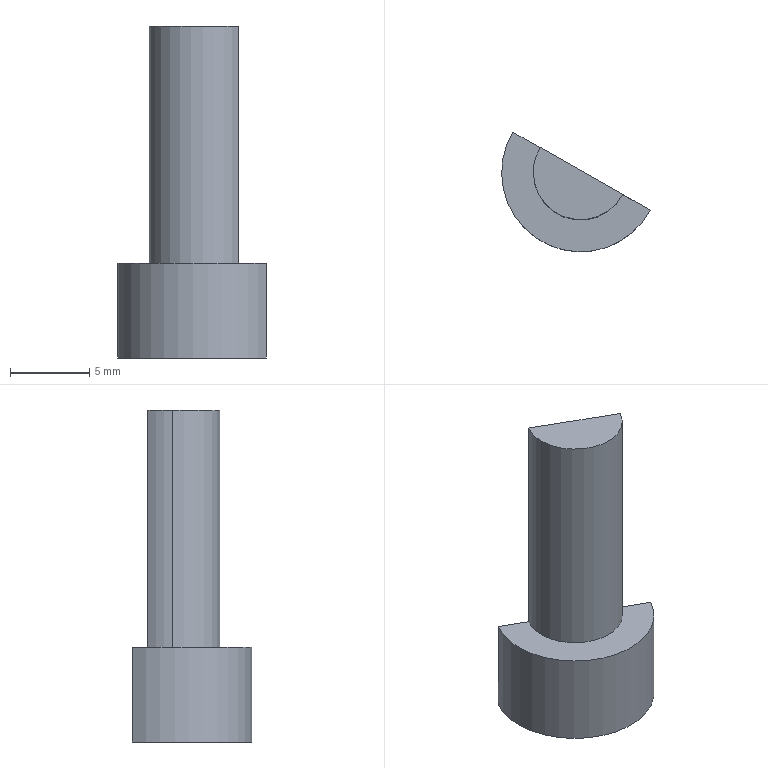Part | STEP file | LG M6_1.5F | 1 solid | 12 faces | box 9.402 x 7.564 x 21 mm | volume 429.881 mm3 | plane 9 | cylinder 3 | commonest cylinder face diameters 6 x2 10 x1
STEP:
#1=CARTESIAN_POINT('',(0.,0.,0.));
#2=DIRECTION('',(0.,0.,1.));
#3=DIRECTION('',(1.,0.,0.));
#4=AXIS2_PLACEMENT_3D('',#1,#2,#3);
#5=CARTESIAN_POINT('',(-3.,0.,15.));
#6=VERTEX_POINT('',#5);
#7=CARTESIAN_POINT('',(2.662,-1.383,15.));
#8=VERTEX_POINT('',#7);
#9=CARTESIAN_POINT('',(0.,0.,15.));
#10=DIRECTION('',(0.,0.,1.));
#11=DIRECTION('',(1.,0.,0.));
#12=AXIS2_PLACEMENT_3D('',#9,#10,#11);
#13=CIRCLE('',#12,3.);
#14=CARTESIAN_POINT('',(0.,0.,15.));
#15=DIRECTION('',(0.,0.,-1.));
#16=DIRECTION('',(-1.,0.,0.));
#17=AXIS2_PLACEMENT_3D('',#14,#15,#16);
#18=CYLINDRICAL_SURFACE('',#17,3.);
#19=CARTESIAN_POINT('',(9.425,0.));
#20=DIRECTION('',(-1.,0.));
#21=VECTOR('',#20,1.);
#22=LINE('',#19,#21);
#23=(GEOMETRIC_REPRESENTATION_CONTEXT(2)PARAMETRIC_REPRESENTATION_CONTEXT()REPRESENTATION_CONTEXT('',''));
#24=DEFINITIONAL_REPRESENTATION('',(#22),#23);
#25=PCURVE('',#18,#24);
#26=CARTESIAN_POINT('',(0.,0.,15.));
#27=DIRECTION('',(0.,0.,1.));
#28=DIRECTION('',(1.,0.,0.));
#29=AXIS2_PLACEMENT_3D('',#26,#27,#28);
#30=PLANE('',#29);
#31=CARTESIAN_POINT('',(0.,0.));
#32=DIRECTION('',(1.,0.));
#33=AXIS2_PLACEMENT_2D('',#31,#32);
#34=CIRCLE('',#33,3.);
#35=(GEOMETRIC_REPRESENTATION_CONTEXT(2)PARAMETRIC_REPRESENTATION_CONTEXT()REPRESENTATION_CONTEXT('',''));
#36=DEFINITIONAL_REPRESENTATION('',(#34),#35);
#37=PCURVE('',#30,#36);
#38=SURFACE_CURVE('',#13,(#25,#37),.PCURVE_S1.);
#39=EDGE_CURVE('',#6,#8,#38,.T.);
#40=ORIENTED_EDGE('',*,*,#39,.F.);
#41=CARTESIAN_POINT('',(-3.,0.,0.));
#42=VERTEX_POINT('',#41);
#43=CARTESIAN_POINT('',(-3.,0.,15.));
#44=DIRECTION('',(0.,0.,-1.));
#45=VECTOR('',#44,1.);
#46=LINE('',#43,#45);
#47=CARTESIAN_POINT('',(6.283,0.));
#48=DIRECTION('',(0.,1.));
#49=VECTOR('',#48,1.);
#50=LINE('',#47,#49);
#51=(GEOMETRIC_REPRESENTATION_CONTEXT(2)PARAMETRIC_REPRESENTATION_CONTEXT()REPRESENTATION_CONTEXT('',''));
#52=DEFINITIONAL_REPRESENTATION('',(#50),#51);
#53=PCURVE('',#18,#52);
#54=CARTESIAN_POINT('',(0.,0.,15.));
#55=DIRECTION('',(0.,0.,-1.));
#56=DIRECTION('',(-1.,0.,0.));
#57=AXIS2_PLACEMENT_3D('',#54,#55,#56);
#58=CYLINDRICAL_SURFACE('',#57,3.);
#59=CARTESIAN_POINT('',(0.,0.));
#60=DIRECTION('',(0.,1.));
#61=VECTOR('',#60,1.);
#62=LINE('',#59,#61);
#63=(GEOMETRIC_REPRESENTATION_CONTEXT(2)PARAMETRIC_REPRESENTATION_CONTEXT()REPRESENTATION_CONTEXT('',''));
#64=DEFINITIONAL_REPRESENTATION('',(#62),#63);
#65=PCURVE('',#58,#64);
#66=SURFACE_CURVE('',#46,(#53,#65),.PCURVE_S1.);
#67=EDGE_CURVE('',#6,#42,#66,.T.);
#68=ORIENTED_EDGE('',*,*,#67,.T.);
#69=CARTESIAN_POINT('',(2.662,-1.383,0.));
#70=VERTEX_POINT('',#69);
#71=CARTESIAN_POINT('',(0.,0.,0.));
#72=DIRECTION('',(0.,0.,1.));
#73=DIRECTION('',(1.,0.,0.));
#74=AXIS2_PLACEMENT_3D('',#71,#72,#73);
#75=CIRCLE('',#74,3.);
#76=CARTESIAN_POINT('',(9.425,15.));
#77=DIRECTION('',(-1.,0.));
#78=VECTOR('',#77,1.);
#79=LINE('',#76,#78);
#80=(GEOMETRIC_REPRESENTATION_CONTEXT(2)PARAMETRIC_REPRESENTATION_CONTEXT()REPRESENTATION_CONTEXT('',''));
#81=DEFINITIONAL_REPRESENTATION('',(#79),#80);
#82=PCURVE('',#18,#81);
#83=CARTESIAN_POINT('',(0.,0.,0.));
#84=DIRECTION('',(0.,0.,1.));
#85=DIRECTION('',(1.,0.,0.));
#86=AXIS2_PLACEMENT_3D('',#83,#84,#85);
#87=PLANE('',#86);
#88=CARTESIAN_POINT('',(0.,0.));
#89=DIRECTION('',(1.,0.));
#90=AXIS2_PLACEMENT_2D('',#88,#89);
#91=CIRCLE('',#90,3.);
#92=(GEOMETRIC_REPRESENTATION_CONTEXT(2)PARAMETRIC_REPRESENTATION_CONTEXT()REPRESENTATION_CONTEXT('',''));
#93=DEFINITIONAL_REPRESENTATION('',(#91),#92);
#94=PCURVE('',#87,#93);
#95=SURFACE_CURVE('',#75,(#82,#94),.PCURVE_S1.);
#96=EDGE_CURVE('',#42,#70,#95,.T.);
#97=ORIENTED_EDGE('',*,*,#96,.T.);
#98=CARTESIAN_POINT('',(2.662,-1.383,15.));
#99=DIRECTION('',(0.,0.,1.));
#100=VECTOR('',#99,1.);
#101=LINE('',#98,#100);
#102=CARTESIAN_POINT('',(3.621,0.));
#103=DIRECTION('',(0.,-1.));
#104=VECTOR('',#103,1.);
#105=LINE('',#102,#104);
#106=(GEOMETRIC_REPRESENTATION_CONTEXT(2)PARAMETRIC_REPRESENTATION_CONTEXT()REPRESENTATION_CONTEXT('',''));
#107=DEFINITIONAL_REPRESENTATION('',(#105),#106);
#108=PCURVE('',#18,#107);
#109=CARTESIAN_POINT('',(312.967,-177.494,-20.57));
#110=DIRECTION('',(-0.4936,-0.8697,0.));
#111=DIRECTION('',(0.8697,-0.4936,0.));
#112=AXIS2_PLACEMENT_3D('',#109,#110,#111);
#113=PLANE('',#112);
#114=CARTESIAN_POINT('',(-356.797,35.57));
#115=DIRECTION('',(0.,1.));
#116=VECTOR('',#115,1.);
#117=LINE('',#114,#116);
#118=(GEOMETRIC_REPRESENTATION_CONTEXT(2)PARAMETRIC_REPRESENTATION_CONTEXT()REPRESENTATION_CONTEXT('',''));
#119=DEFINITIONAL_REPRESENTATION('',(#117),#118);
#120=PCURVE('',#113,#119);
#121=SURFACE_CURVE('',#101,(#108,#120),.PCURVE_S1.);
#122=EDGE_CURVE('',#70,#8,#121,.T.);
#123=ORIENTED_EDGE('',*,*,#122,.T.);
#124=EDGE_LOOP('',(#40,#68,#97,#123));
#125=FACE_BOUND('',#124,.T.);
#126=ADVANCED_FACE('',(#125),#18,.T.);
#127=CARTESIAN_POINT('',(-4.293,2.564,0.));
#128=VERTEX_POINT('',#127);
#129=CARTESIAN_POINT('',(-2.553,1.576,0.));
#130=VERTEX_POINT('',#129);
#131=CARTESIAN_POINT('',(0.05466,0.09631,0.));
#132=DIRECTION('',(0.8697,-0.4936,0.));
#133=VECTOR('',#132,1.);
#134=LINE('',#131,#133);
#135=CARTESIAN_POINT('',(0.05466,0.09631));
#136=DIRECTION('',(0.8697,-0.4936));
#137=VECTOR('',#136,1.);
#138=LINE('',#135,#137);
#139=(GEOMETRIC_REPRESENTATION_CONTEXT(2)PARAMETRIC_REPRESENTATION_CONTEXT()REPRESENTATION_CONTEXT('',''));
#140=DEFINITIONAL_REPRESENTATION('',(#138),#139);
#141=PCURVE('',#87,#140);
#142=CARTESIAN_POINT('',(-359.795,20.57));
#143=DIRECTION('',(1.,0.));
#144=VECTOR('',#143,1.);
#145=LINE('',#142,#144);
#146=(GEOMETRIC_REPRESENTATION_CONTEXT(2)PARAMETRIC_REPRESENTATION_CONTEXT()REPRESENTATION_CONTEXT('',''));
#147=DEFINITIONAL_REPRESENTATION('',(#145),#146);
#148=PCURVE('',#113,#147);
#149=SURFACE_CURVE('',#134,(#141,#148),.PCURVE_S1.);
#150=EDGE_CURVE('',#128,#130,#149,.T.);
#151=ORIENTED_EDGE('',*,*,#150,.F.);
#152=CARTESIAN_POINT('',(4.402,-2.371,0.));
#153=VERTEX_POINT('',#152);
#154=CARTESIAN_POINT('',(0.,0.,0.));
#155=DIRECTION('',(0.,0.,1.));
#156=DIRECTION('',(1.,0.,0.));
#157=AXIS2_PLACEMENT_3D('',#154,#155,#156);
#158=CIRCLE('',#157,5.);
#159=CARTESIAN_POINT('',(0.,0.));
#160=DIRECTION('',(1.,0.));
#161=AXIS2_PLACEMENT_2D('',#159,#160);
#162=CIRCLE('',#161,5.);
#163=(GEOMETRIC_REPRESENTATION_CONTEXT(2)PARAMETRIC_REPRESENTATION_CONTEXT()REPRESENTATION_CONTEXT('',''));
#164=DEFINITIONAL_REPRESENTATION('',(#162),#163);
#165=PCURVE('',#87,#164);
#166=CARTESIAN_POINT('',(0.,0.,-6.));
#167=DIRECTION('',(0.,0.,1.));
#168=DIRECTION('',(1.,0.,0.));
#169=AXIS2_PLACEMENT_3D('',#166,#167,#168);
#170=CYLINDRICAL_SURFACE('',#169,5.);
#171=CARTESIAN_POINT('',(0.,6.));
#172=DIRECTION('',(1.,0.));
#173=VECTOR('',#172,1.);
#174=LINE('',#171,#173);
#175=(GEOMETRIC_REPRESENTATION_CONTEXT(2)PARAMETRIC_REPRESENTATION_CONTEXT()REPRESENTATION_CONTEXT('',''));
#176=DEFINITIONAL_REPRESENTATION('',(#174),#175);
#177=PCURVE('',#170,#176);
#178=SURFACE_CURVE('',#158,(#165,#177),.PCURVE_S1.);
#179=EDGE_CURVE('',#128,#153,#178,.T.);
#180=ORIENTED_EDGE('',*,*,#179,.T.);
#181=CARTESIAN_POINT('',(0.05466,0.09631,0.));
#182=DIRECTION('',(0.8697,-0.4936,0.));
#183=VECTOR('',#182,1.);
#184=LINE('',#181,#183);
#185=CARTESIAN_POINT('',(0.05466,0.09631));
#186=DIRECTION('',(0.8697,-0.4936));
#187=VECTOR('',#186,1.);
#188=LINE('',#185,#187);
#189=(GEOMETRIC_REPRESENTATION_CONTEXT(2)PARAMETRIC_REPRESENTATION_CONTEXT()REPRESENTATION_CONTEXT('',''));
#190=DEFINITIONAL_REPRESENTATION('',(#188),#189);
#191=PCURVE('',#87,#190);
#192=CARTESIAN_POINT('',(-359.795,20.57));
#193=DIRECTION('',(1.,0.));
#194=VECTOR('',#193,1.);
#195=LINE('',#192,#194);
#196=(GEOMETRIC_REPRESENTATION_CONTEXT(2)PARAMETRIC_REPRESENTATION_CONTEXT()REPRESENTATION_CONTEXT('',''));
#197=DEFINITIONAL_REPRESENTATION('',(#195),#196);
#198=PCURVE('',#113,#197);
#199=SURFACE_CURVE('',#184,(#191,#198),.PCURVE_S1.);
#200=EDGE_CURVE('',#70,#153,#199,.T.);
#201=ORIENTED_EDGE('',*,*,#200,.F.);
#202=ORIENTED_EDGE('',*,*,#96,.F.);
#203=CARTESIAN_POINT('',(0.,0.,0.));
#204=DIRECTION('',(0.,0.,1.));
#205=DIRECTION('',(1.,0.,0.));
#206=AXIS2_PLACEMENT_3D('',#203,#204,#205);
#207=CIRCLE('',#206,3.);
#208=CARTESIAN_POINT('',(0.,0.));
#209=DIRECTION('',(1.,0.));
#210=AXIS2_PLACEMENT_2D('',#208,#209);
#211=CIRCLE('',#210,3.);
#212=(GEOMETRIC_REPRESENTATION_CONTEXT(2)PARAMETRIC_REPRESENTATION_CONTEXT()REPRESENTATION_CONTEXT('',''));
#213=DEFINITIONAL_REPRESENTATION('',(#211),#212);
#214=PCURVE('',#87,#213);
#215=CARTESIAN_POINT('',(3.142,15.));
#216=DIRECTION('',(-1.,0.));
#217=VECTOR('',#216,1.);
#218=LINE('',#215,#217);
#219=(GEOMETRIC_REPRESENTATION_CONTEXT(2)PARAMETRIC_REPRESENTATION_CONTEXT()REPRESENTATION_CONTEXT('',''));
#220=DEFINITIONAL_REPRESENTATION('',(#218),#219);
#221=PCURVE('',#58,#220);
#222=SURFACE_CURVE('',#207,(#214,#221),.PCURVE_S1.);
#223=EDGE_CURVE('',#130,#42,#222,.T.);
#224=ORIENTED_EDGE('',*,*,#223,.F.);
#225=EDGE_LOOP('',(#151,#180,#201,#202,#224));
#226=FACE_BOUND('',#225,.T.);
#227=ADVANCED_FACE('',(#226),#87,.T.);
#228=CARTESIAN_POINT('',(4.402,-2.371,-6.));
#229=VERTEX_POINT('',#228);
#230=CARTESIAN_POINT('',(4.402,-2.371,-6.));
#231=DIRECTION('',(0.,0.,-1.));
#232=VECTOR('',#231,1.);
#233=LINE('',#230,#232);
#234=CARTESIAN_POINT('',(5.789,0.));
#235=DIRECTION('',(0.,-1.));
#236=VECTOR('',#235,1.);
#237=LINE('',#234,#236);
#238=(GEOMETRIC_REPRESENTATION_CONTEXT(2)PARAMETRIC_REPRESENTATION_CONTEXT()REPRESENTATION_CONTEXT('',''));
#239=DEFINITIONAL_REPRESENTATION('',(#237),#238);
#240=PCURVE('',#170,#239);
#241=CARTESIAN_POINT('',(-354.796,14.57));
#242=DIRECTION('',(0.,-1.));
#243=VECTOR('',#242,1.);
#244=LINE('',#241,#243);
#245=(GEOMETRIC_REPRESENTATION_CONTEXT(2)PARAMETRIC_REPRESENTATION_CONTEXT()REPRESENTATION_CONTEXT('',''));
#246=DEFINITIONAL_REPRESENTATION('',(#244),#245);
#247=PCURVE('',#113,#246);
#248=SURFACE_CURVE('',#233,(#240,#247),.PCURVE_S1.);
#249=EDGE_CURVE('',#153,#229,#248,.T.);
#250=ORIENTED_EDGE('',*,*,#249,.F.);
#251=ORIENTED_EDGE('',*,*,#179,.F.);
#252=CARTESIAN_POINT('',(-4.293,2.564,-6.));
#253=VERTEX_POINT('',#252);
#254=CARTESIAN_POINT('',(-4.293,2.564,-6.));
#255=DIRECTION('',(0.,0.,1.));
#256=VECTOR('',#255,1.);
#257=LINE('',#254,#256);
#258=CARTESIAN_POINT('',(2.603,0.));
#259=DIRECTION('',(0.,1.));
#260=VECTOR('',#259,1.);
#261=LINE('',#258,#260);
#262=(GEOMETRIC_REPRESENTATION_CONTEXT(2)PARAMETRIC_REPRESENTATION_CONTEXT()REPRESENTATION_CONTEXT('',''));
#263=DEFINITIONAL_REPRESENTATION('',(#261),#262);
#264=PCURVE('',#170,#263);
#265=CARTESIAN_POINT('',(-364.794,14.57));
#266=DIRECTION('',(0.,1.));
#267=VECTOR('',#266,1.);
#268=LINE('',#265,#267);
#269=(GEOMETRIC_REPRESENTATION_CONTEXT(2)PARAMETRIC_REPRESENTATION_CONTEXT()REPRESENTATION_CONTEXT('',''));
#270=DEFINITIONAL_REPRESENTATION('',(#268),#269);
#271=PCURVE('',#113,#270);
#272=SURFACE_CURVE('',#257,(#264,#271),.PCURVE_S1.);
#273=EDGE_CURVE('',#253,#128,#272,.T.);
#274=ORIENTED_EDGE('',*,*,#273,.F.);
#275=CARTESIAN_POINT('',(0.,0.,-6.));
#276=DIRECTION('',(0.,0.,1.));
#277=DIRECTION('',(1.,0.,0.));
#278=AXIS2_PLACEMENT_3D('',#275,#276,#277);
#279=CIRCLE('',#278,5.);
#280=CARTESIAN_POINT('',(0.,0.));
#281=DIRECTION('',(1.,0.));
#282=VECTOR('',#281,1.);
#283=LINE('',#280,#282);
#284=(GEOMETRIC_REPRESENTATION_CONTEXT(2)PARAMETRIC_REPRESENTATION_CONTEXT()REPRESENTATION_CONTEXT('',''));
#285=DEFINITIONAL_REPRESENTATION('',(#283),#284);
#286=PCURVE('',#170,#285);
#287=CARTESIAN_POINT('',(0.,0.,-6.));
#288=DIRECTION('',(0.,0.,1.));
#289=DIRECTION('',(1.,0.,0.));
#290=AXIS2_PLACEMENT_3D('',#287,#288,#289);
#291=PLANE('',#290);
#292=CARTESIAN_POINT('',(0.,0.));
#293=DIRECTION('',(1.,0.));
#294=AXIS2_PLACEMENT_2D('',#292,#293);
#295=CIRCLE('',#294,5.);
#296=(GEOMETRIC_REPRESENTATION_CONTEXT(2)PARAMETRIC_REPRESENTATION_CONTEXT()REPRESENTATION_CONTEXT('',''));
#297=DEFINITIONAL_REPRESENTATION('',(#295),#296);
#298=PCURVE('',#291,#297);
#299=SURFACE_CURVE('',#279,(#286,#298),.PCURVE_S1.);
#300=EDGE_CURVE('',#253,#229,#299,.T.);
#301=ORIENTED_EDGE('',*,*,#300,.T.);
#302=EDGE_LOOP('',(#250,#251,#274,#301));
#303=FACE_BOUND('',#302,.T.);
#304=ADVANCED_FACE('',(#303),#170,.T.);
#305=ORIENTED_EDGE('',*,*,#300,.F.);
#306=CARTESIAN_POINT('',(-2.128,1.335,-6.));
#307=VERTEX_POINT('',#306);
#308=CARTESIAN_POINT('',(0.05466,0.09631,-6.));
#309=DIRECTION('',(0.8697,-0.4936,0.));
#310=VECTOR('',#309,1.);
#311=LINE('',#308,#310);
#312=CARTESIAN_POINT('',(0.05466,0.09631));
#313=DIRECTION('',(0.8697,-0.4936));
#314=VECTOR('',#313,1.);
#315=LINE('',#312,#314);
#316=(GEOMETRIC_REPRESENTATION_CONTEXT(2)PARAMETRIC_REPRESENTATION_CONTEXT()REPRESENTATION_CONTEXT('',''));
#317=DEFINITIONAL_REPRESENTATION('',(#315),#316);
#318=PCURVE('',#291,#317);
#319=CARTESIAN_POINT('',(-359.795,14.57));
#320=DIRECTION('',(1.,0.));
#321=VECTOR('',#320,1.);
#322=LINE('',#319,#321);
#323=(GEOMETRIC_REPRESENTATION_CONTEXT(2)PARAMETRIC_REPRESENTATION_CONTEXT()REPRESENTATION_CONTEXT('',''));
#324=DEFINITIONAL_REPRESENTATION('',(#322),#323);
#325=PCURVE('',#113,#324);
#326=SURFACE_CURVE('',#311,(#318,#325),.PCURVE_S1.);
#327=EDGE_CURVE('',#253,#307,#326,.T.);
#328=ORIENTED_EDGE('',*,*,#327,.T.);
#329=CARTESIAN_POINT('',(-2.898,0.,-6.));
#330=VERTEX_POINT('',#329);
#331=CARTESIAN_POINT('',(-2.898,0.,-6.));
#332=DIRECTION('',(0.5,0.866,0.));
#333=VECTOR('',#332,1.);
#334=LINE('',#331,#333);
#335=CARTESIAN_POINT('',(-2.898,0.));
#336=DIRECTION('',(0.5,0.866));
#337=VECTOR('',#336,1.);
#338=LINE('',#335,#337);
#339=(GEOMETRIC_REPRESENTATION_CONTEXT(2)PARAMETRIC_REPRESENTATION_CONTEXT()REPRESENTATION_CONTEXT('',''));
#340=DEFINITIONAL_REPRESENTATION('',(#338),#339);
#341=PCURVE('',#291,#340);
#342=CARTESIAN_POINT('',(-2.898,0.,-3.));
#343=DIRECTION('',(-0.866,0.5,0.));
#344=DIRECTION('',(-0.5,-0.866,0.));
#345=AXIS2_PLACEMENT_3D('',#342,#343,#344);
#346=PLANE('',#345);
#347=CARTESIAN_POINT('',(0.,-3.));
#348=DIRECTION('',(-1.,0.));
#349=VECTOR('',#348,1.);
#350=LINE('',#347,#349);
#351=(GEOMETRIC_REPRESENTATION_CONTEXT(2)PARAMETRIC_REPRESENTATION_CONTEXT()REPRESENTATION_CONTEXT('',''));
#352=DEFINITIONAL_REPRESENTATION('',(#350),#351);
#353=PCURVE('',#346,#352);
#354=SURFACE_CURVE('',#334,(#341,#353),.PCURVE_S1.);
#355=EDGE_CURVE('',#330,#307,#354,.T.);
#356=ORIENTED_EDGE('',*,*,#355,.F.);
#357=CARTESIAN_POINT('',(-1.449,-2.51,-6.));
#358=VERTEX_POINT('',#357);
#359=CARTESIAN_POINT('',(-1.449,-2.51,-6.));
#360=DIRECTION('',(-0.5,0.866,0.));
#361=VECTOR('',#360,1.);
#362=LINE('',#359,#361);
#363=CARTESIAN_POINT('',(-1.449,-2.51));
#364=DIRECTION('',(-0.5,0.866));
#365=VECTOR('',#364,1.);
#366=LINE('',#363,#365);
#367=(GEOMETRIC_REPRESENTATION_CONTEXT(2)PARAMETRIC_REPRESENTATION_CONTEXT()REPRESENTATION_CONTEXT('',''));
#368=DEFINITIONAL_REPRESENTATION('',(#366),#367);
#369=PCURVE('',#291,#368);
#370=CARTESIAN_POINT('',(-1.449,-2.51,-3.));
#371=DIRECTION('',(-0.866,-0.5,0.));
#372=DIRECTION('',(0.5,-0.866,0.));
#373=AXIS2_PLACEMENT_3D('',#370,#371,#372);
#374=PLANE('',#373);
#375=CARTESIAN_POINT('',(0.,-3.));
#376=DIRECTION('',(-1.,0.));
#377=VECTOR('',#376,1.);
#378=LINE('',#375,#377);
#379=(GEOMETRIC_REPRESENTATION_CONTEXT(2)PARAMETRIC_REPRESENTATION_CONTEXT()REPRESENTATION_CONTEXT('',''));
#380=DEFINITIONAL_REPRESENTATION('',(#378),#379);
#381=PCURVE('',#374,#380);
#382=SURFACE_CURVE('',#362,(#369,#381),.PCURVE_S1.);
#383=EDGE_CURVE('',#358,#330,#382,.T.);
#384=ORIENTED_EDGE('',*,*,#383,.F.);
#385=CARTESIAN_POINT('',(1.449,-2.51,-6.));
#386=VERTEX_POINT('',#385);
#387=CARTESIAN_POINT('',(1.449,-2.51,-6.));
#388=DIRECTION('',(-1.,0.,0.));
#389=VECTOR('',#388,1.);
#390=LINE('',#387,#389);
#391=CARTESIAN_POINT('',(1.449,-2.51));
#392=DIRECTION('',(-1.,0.));
#393=VECTOR('',#392,1.);
#394=LINE('',#391,#393);
#395=(GEOMETRIC_REPRESENTATION_CONTEXT(2)PARAMETRIC_REPRESENTATION_CONTEXT()REPRESENTATION_CONTEXT('',''));
#396=DEFINITIONAL_REPRESENTATION('',(#394),#395);
#397=PCURVE('',#291,#396);
#398=CARTESIAN_POINT('',(1.449,-2.51,-3.));
#399=DIRECTION('',(0.,-1.,0.));
#400=DIRECTION('',(0.,0.,-1.));
#401=AXIS2_PLACEMENT_3D('',#398,#399,#400);
#402=PLANE('',#401);
#403=CARTESIAN_POINT('',(3.,0.));
#404=DIRECTION('',(0.,-1.));
#405=VECTOR('',#404,1.);
#406=LINE('',#403,#405);
#407=(GEOMETRIC_REPRESENTATION_CONTEXT(2)PARAMETRIC_REPRESENTATION_CONTEXT()REPRESENTATION_CONTEXT('',''));
#408=DEFINITIONAL_REPRESENTATION('',(#406),#407);
#409=PCURVE('',#402,#408);
#410=SURFACE_CURVE('',#390,(#397,#409),.PCURVE_S1.);
#411=EDGE_CURVE('',#386,#358,#410,.T.);
#412=ORIENTED_EDGE('',*,*,#411,.F.);
#413=CARTESIAN_POINT('',(2.238,-1.143,-6.));
#414=VERTEX_POINT('',#413);
#415=CARTESIAN_POINT('',(2.898,0.,-6.));
#416=DIRECTION('',(-0.5,-0.866,0.));
#417=VECTOR('',#416,1.);
#418=LINE('',#415,#417);
#419=CARTESIAN_POINT('',(2.898,0.));
#420=DIRECTION('',(-0.5,-0.866));
#421=VECTOR('',#420,1.);
#422=LINE('',#419,#421);
#423=(GEOMETRIC_REPRESENTATION_CONTEXT(2)PARAMETRIC_REPRESENTATION_CONTEXT()REPRESENTATION_CONTEXT('',''));
#424=DEFINITIONAL_REPRESENTATION('',(#422),#423);
#425=PCURVE('',#291,#424);
#426=CARTESIAN_POINT('',(2.898,0.,-3.));
#427=DIRECTION('',(0.866,-0.5,0.));
#428=DIRECTION('',(0.5,0.866,0.));
#429=AXIS2_PLACEMENT_3D('',#426,#427,#428);
#430=PLANE('',#429);
#431=CARTESIAN_POINT('',(0.,-3.));
#432=DIRECTION('',(-1.,0.));
#433=VECTOR('',#432,1.);
#434=LINE('',#431,#433);
#435=(GEOMETRIC_REPRESENTATION_CONTEXT(2)PARAMETRIC_REPRESENTATION_CONTEXT()REPRESENTATION_CONTEXT('',''));
#436=DEFINITIONAL_REPRESENTATION('',(#434),#435);
#437=PCURVE('',#430,#436);
#438=SURFACE_CURVE('',#418,(#425,#437),.PCURVE_S1.);
#439=EDGE_CURVE('',#414,#386,#438,.T.);
#440=ORIENTED_EDGE('',*,*,#439,.F.);
#441=CARTESIAN_POINT('',(0.05466,0.09631,-6.));
#442=DIRECTION('',(0.8697,-0.4936,0.));
#443=VECTOR('',#442,1.);
#444=LINE('',#441,#443);
#445=CARTESIAN_POINT('',(0.05466,0.09631));
#446=DIRECTION('',(0.8697,-0.4936));
#447=VECTOR('',#446,1.);
#448=LINE('',#445,#447);
#449=(GEOMETRIC_REPRESENTATION_CONTEXT(2)PARAMETRIC_REPRESENTATION_CONTEXT()REPRESENTATION_CONTEXT('',''));
#450=DEFINITIONAL_REPRESENTATION('',(#448),#449);
#451=PCURVE('',#291,#450);
#452=CARTESIAN_POINT('',(-359.795,14.57));
#453=DIRECTION('',(1.,0.));
#454=VECTOR('',#453,1.);
#455=LINE('',#452,#454);
#456=(GEOMETRIC_REPRESENTATION_CONTEXT(2)PARAMETRIC_REPRESENTATION_CONTEXT()REPRESENTATION_CONTEXT('',''));
#457=DEFINITIONAL_REPRESENTATION('',(#455),#456);
#458=PCURVE('',#113,#457);
#459=SURFACE_CURVE('',#444,(#451,#458),.PCURVE_S1.);
#460=EDGE_CURVE('',#414,#229,#459,.T.);
#461=ORIENTED_EDGE('',*,*,#460,.T.);
#462=EDGE_LOOP('',(#305,#328,#356,#384,#412,#440,#461));
#463=FACE_BOUND('',#462,.T.);
#464=ADVANCED_FACE('',(#463),#291,.F.);
#465=ORIENTED_EDGE('',*,*,#67,.F.);
#466=CARTESIAN_POINT('',(-2.553,1.576,15.));
#467=VERTEX_POINT('',#466);
#468=CARTESIAN_POINT('',(0.,0.,15.));
#469=DIRECTION('',(0.,0.,1.));
#470=DIRECTION('',(1.,0.,0.));
#471=AXIS2_PLACEMENT_3D('',#468,#469,#470);
#472=CIRCLE('',#471,3.);
#473=CARTESIAN_POINT('',(3.142,0.));
#474=DIRECTION('',(-1.,0.));
#475=VECTOR('',#474,1.);
#476=LINE('',#473,#475);
#477=(GEOMETRIC_REPRESENTATION_CONTEXT(2)PARAMETRIC_REPRESENTATION_CONTEXT()REPRESENTATION_CONTEXT('',''));
#478=DEFINITIONAL_REPRESENTATION('',(#476),#477);
#479=PCURVE('',#58,#478);
#480=CARTESIAN_POINT('',(0.,0.));
#481=DIRECTION('',(1.,0.));
#482=AXIS2_PLACEMENT_2D('',#480,#481);
#483=CIRCLE('',#482,3.);
#484=(GEOMETRIC_REPRESENTATION_CONTEXT(2)PARAMETRIC_REPRESENTATION_CONTEXT()REPRESENTATION_CONTEXT('',''));
#485=DEFINITIONAL_REPRESENTATION('',(#483),#484);
#486=PCURVE('',#30,#485);
#487=SURFACE_CURVE('',#472,(#479,#486),.PCURVE_S1.);
#488=EDGE_CURVE('',#467,#6,#487,.T.);
#489=ORIENTED_EDGE('',*,*,#488,.F.);
#490=CARTESIAN_POINT('',(-2.553,1.576,15.));
#491=DIRECTION('',(0.,0.,-1.));
#492=VECTOR('',#491,1.);
#493=LINE('',#490,#492);
#494=CARTESIAN_POINT('',(0.5531,0.));
#495=DIRECTION('',(0.,1.));
#496=VECTOR('',#495,1.);
#497=LINE('',#494,#496);
#498=(GEOMETRIC_REPRESENTATION_CONTEXT(2)PARAMETRIC_REPRESENTATION_CONTEXT()REPRESENTATION_CONTEXT('',''));
#499=DEFINITIONAL_REPRESENTATION('',(#497),#498);
#500=PCURVE('',#58,#499);
#501=CARTESIAN_POINT('',(-362.793,35.57));
#502=DIRECTION('',(0.,-1.));
#503=VECTOR('',#502,1.);
#504=LINE('',#501,#503);
#505=(GEOMETRIC_REPRESENTATION_CONTEXT(2)PARAMETRIC_REPRESENTATION_CONTEXT()REPRESENTATION_CONTEXT('',''));
#506=DEFINITIONAL_REPRESENTATION('',(#504),#505);
#507=PCURVE('',#113,#506);
#508=SURFACE_CURVE('',#493,(#500,#507),.PCURVE_S1.);
#509=EDGE_CURVE('',#467,#130,#508,.T.);
#510=ORIENTED_EDGE('',*,*,#509,.T.);
#511=ORIENTED_EDGE('',*,*,#223,.T.);
#512=EDGE_LOOP('',(#465,#489,#510,#511));
#513=FACE_BOUND('',#512,.T.);
#514=ADVANCED_FACE('',(#513),#58,.T.);
#515=CARTESIAN_POINT('',(0.05466,0.09631,15.));
#516=DIRECTION('',(0.8697,-0.4936,0.));
#517=VECTOR('',#516,1.);
#518=LINE('',#515,#517);
#519=CARTESIAN_POINT('',(0.05466,0.09631));
#520=DIRECTION('',(0.8697,-0.4936));
#521=VECTOR('',#520,1.);
#522=LINE('',#519,#521);
#523=(GEOMETRIC_REPRESENTATION_CONTEXT(2)PARAMETRIC_REPRESENTATION_CONTEXT()REPRESENTATION_CONTEXT('',''));
#524=DEFINITIONAL_REPRESENTATION('',(#522),#523);
#525=PCURVE('',#30,#524);
#526=CARTESIAN_POINT('',(-359.795,35.57));
#527=DIRECTION('',(1.,0.));
#528=VECTOR('',#527,1.);
#529=LINE('',#526,#528);
#530=(GEOMETRIC_REPRESENTATION_CONTEXT(2)PARAMETRIC_REPRESENTATION_CONTEXT()REPRESENTATION_CONTEXT('',''));
#531=DEFINITIONAL_REPRESENTATION('',(#529),#530);
#532=PCURVE('',#113,#531);
#533=SURFACE_CURVE('',#518,(#525,#532),.PCURVE_S1.);
#534=EDGE_CURVE('',#467,#8,#533,.T.);
#535=ORIENTED_EDGE('',*,*,#534,.F.);
#536=ORIENTED_EDGE('',*,*,#488,.T.);
#537=ORIENTED_EDGE('',*,*,#39,.T.);
#538=EDGE_LOOP('',(#535,#536,#537));
#539=FACE_BOUND('',#538,.T.);
#540=ADVANCED_FACE('',(#539),#30,.T.);
#541=ORIENTED_EDGE('',*,*,#383,.T.);
#542=CARTESIAN_POINT('',(-2.898,0.,-3.));
#543=VERTEX_POINT('',#542);
#544=CARTESIAN_POINT('',(-2.898,0.,-3.));
#545=DIRECTION('',(0.,0.,-1.));
#546=VECTOR('',#545,1.);
#547=LINE('',#544,#546);
#548=CARTESIAN_POINT('',(-2.898,0.));
#549=DIRECTION('',(0.,-1.));
#550=VECTOR('',#549,1.);
#551=LINE('',#548,#550);
#552=(GEOMETRIC_REPRESENTATION_CONTEXT(2)PARAMETRIC_REPRESENTATION_CONTEXT()REPRESENTATION_CONTEXT('',''));
#553=DEFINITIONAL_REPRESENTATION('',(#551),#552);
#554=PCURVE('',#374,#553);
#555=CARTESIAN_POINT('',(0.,0.));
#556=DIRECTION('',(0.,-1.));
#557=VECTOR('',#556,1.);
#558=LINE('',#555,#557);
#559=(GEOMETRIC_REPRESENTATION_CONTEXT(2)PARAMETRIC_REPRESENTATION_CONTEXT()REPRESENTATION_CONTEXT('',''));
#560=DEFINITIONAL_REPRESENTATION('',(#558),#559);
#561=PCURVE('',#346,#560);
#562=SURFACE_CURVE('',#547,(#554,#561),.PCURVE_S1.);
#563=EDGE_CURVE('',#543,#330,#562,.T.);
#564=ORIENTED_EDGE('',*,*,#563,.F.);
#565=CARTESIAN_POINT('',(-1.449,-2.51,-3.));
#566=VERTEX_POINT('',#565);
#567=CARTESIAN_POINT('',(-1.449,-2.51,-3.));
#568=DIRECTION('',(-0.5,0.866,0.));
#569=VECTOR('',#568,1.);
#570=LINE('',#567,#569);
#571=CARTESIAN_POINT('',(0.,0.));
#572=DIRECTION('',(-1.,0.));
#573=VECTOR('',#572,1.);
#574=LINE('',#571,#573);
#575=(GEOMETRIC_REPRESENTATION_CONTEXT(2)PARAMETRIC_REPRESENTATION_CONTEXT()REPRESENTATION_CONTEXT('',''));
#576=DEFINITIONAL_REPRESENTATION('',(#574),#575);
#577=PCURVE('',#374,#576);
#578=CARTESIAN_POINT('',(0.,0.,-3.));
#579=DIRECTION('',(0.,0.,-1.));
#580=DIRECTION('',(-1.,0.,0.));
#581=AXIS2_PLACEMENT_3D('',#578,#579,#580);
#582=PLANE('',#581);
#583=CARTESIAN_POINT('',(1.449,-2.51));
#584=DIRECTION('',(0.5,0.866));
#585=VECTOR('',#584,1.);
#586=LINE('',#583,#585);
#587=(GEOMETRIC_REPRESENTATION_CONTEXT(2)PARAMETRIC_REPRESENTATION_CONTEXT()REPRESENTATION_CONTEXT('',''));
#588=DEFINITIONAL_REPRESENTATION('',(#586),#587);
#589=PCURVE('',#582,#588);
#590=SURFACE_CURVE('',#570,(#577,#589),.PCURVE_S1.);
#591=EDGE_CURVE('',#566,#543,#590,.T.);
#592=ORIENTED_EDGE('',*,*,#591,.F.);
#593=CARTESIAN_POINT('',(-1.449,-2.51,-3.));
#594=DIRECTION('',(0.,0.,-1.));
#595=VECTOR('',#594,1.);
#596=LINE('',#593,#595);
#597=CARTESIAN_POINT('',(0.,0.));
#598=DIRECTION('',(0.,-1.));
#599=VECTOR('',#598,1.);
#600=LINE('',#597,#599);
#601=(GEOMETRIC_REPRESENTATION_CONTEXT(2)PARAMETRIC_REPRESENTATION_CONTEXT()REPRESENTATION_CONTEXT('',''));
#602=DEFINITIONAL_REPRESENTATION('',(#600),#601);
#603=PCURVE('',#374,#602);
#604=CARTESIAN_POINT('',(0.,-2.898));
#605=DIRECTION('',(1.,0.));
#606=VECTOR('',#605,1.);
#607=LINE('',#604,#606);
#608=(GEOMETRIC_REPRESENTATION_CONTEXT(2)PARAMETRIC_REPRESENTATION_CONTEXT()REPRESENTATION_CONTEXT('',''));
#609=DEFINITIONAL_REPRESENTATION('',(#607),#608);
#610=PCURVE('',#402,#609);
#611=SURFACE_CURVE('',#596,(#603,#610),.PCURVE_S1.);
#612=EDGE_CURVE('',#566,#358,#611,.T.);
#613=ORIENTED_EDGE('',*,*,#612,.T.);
#614=EDGE_LOOP('',(#541,#564,#592,#613));
#615=FACE_BOUND('',#614,.T.);
#616=ADVANCED_FACE('',(#615),#374,.F.);
#617=ORIENTED_EDGE('',*,*,#411,.T.);
#618=ORIENTED_EDGE('',*,*,#612,.F.);
#619=CARTESIAN_POINT('',(1.449,-2.51,-3.));
#620=VERTEX_POINT('',#619);
#621=CARTESIAN_POINT('',(1.449,-2.51,-3.));
#622=DIRECTION('',(-1.,0.,0.));
#623=VECTOR('',#622,1.);
#624=LINE('',#621,#623);
#625=CARTESIAN_POINT('',(0.,0.));
#626=DIRECTION('',(0.,-1.));
#627=VECTOR('',#626,1.);
#628=LINE('',#625,#627);
#629=(GEOMETRIC_REPRESENTATION_CONTEXT(2)PARAMETRIC_REPRESENTATION_CONTEXT()REPRESENTATION_CONTEXT('',''));
#630=DEFINITIONAL_REPRESENTATION('',(#628),#629);
#631=PCURVE('',#402,#630);
#632=CARTESIAN_POINT('',(-1.449,-2.51));
#633=DIRECTION('',(1.,0.));
#634=VECTOR('',#633,1.);
#635=LINE('',#632,#634);
#636=(GEOMETRIC_REPRESENTATION_CONTEXT(2)PARAMETRIC_REPRESENTATION_CONTEXT()REPRESENTATION_CONTEXT('',''));
#637=DEFINITIONAL_REPRESENTATION('',(#635),#636);
#638=PCURVE('',#582,#637);
#639=SURFACE_CURVE('',#624,(#631,#638),.PCURVE_S1.);
#640=EDGE_CURVE('',#620,#566,#639,.T.);
#641=ORIENTED_EDGE('',*,*,#640,.F.);
#642=CARTESIAN_POINT('',(1.449,-2.51,-3.));
#643=DIRECTION('',(0.,0.,-1.));
#644=VECTOR('',#643,1.);
#645=LINE('',#642,#644);
#646=CARTESIAN_POINT('',(0.,0.));
#647=DIRECTION('',(1.,0.));
#648=VECTOR('',#647,1.);
#649=LINE('',#646,#648);
#650=(GEOMETRIC_REPRESENTATION_CONTEXT(2)PARAMETRIC_REPRESENTATION_CONTEXT()REPRESENTATION_CONTEXT('',''));
#651=DEFINITIONAL_REPRESENTATION('',(#649),#650);
#652=PCURVE('',#402,#651);
#653=CARTESIAN_POINT('',(-2.898,0.));
#654=DIRECTION('',(0.,-1.));
#655=VECTOR('',#654,1.);
#656=LINE('',#653,#655);
#657=(GEOMETRIC_REPRESENTATION_CONTEXT(2)PARAMETRIC_REPRESENTATION_CONTEXT()REPRESENTATION_CONTEXT('',''));
#658=DEFINITIONAL_REPRESENTATION('',(#656),#657);
#659=PCURVE('',#430,#658);
#660=SURFACE_CURVE('',#645,(#652,#659),.PCURVE_S1.);
#661=EDGE_CURVE('',#620,#386,#660,.T.);
#662=ORIENTED_EDGE('',*,*,#661,.T.);
#663=EDGE_LOOP('',(#617,#618,#641,#662));
#664=FACE_BOUND('',#663,.T.);
#665=ADVANCED_FACE('',(#664),#402,.F.);
#666=CARTESIAN_POINT('',(2.238,-1.143,-3.));
#667=VERTEX_POINT('',#666);
#668=CARTESIAN_POINT('',(2.898,0.,-3.));
#669=DIRECTION('',(-0.5,-0.866,0.));
#670=VECTOR('',#669,1.);
#671=LINE('',#668,#670);
#672=CARTESIAN_POINT('',(0.,0.));
#673=DIRECTION('',(-1.,0.));
#674=VECTOR('',#673,1.);
#675=LINE('',#672,#674);
#676=(GEOMETRIC_REPRESENTATION_CONTEXT(2)PARAMETRIC_REPRESENTATION_CONTEXT()REPRESENTATION_CONTEXT('',''));
#677=DEFINITIONAL_REPRESENTATION('',(#675),#676);
#678=PCURVE('',#430,#677);
#679=CARTESIAN_POINT('',(-2.898,0.));
#680=DIRECTION('',(0.5,-0.866));
#681=VECTOR('',#680,1.);
#682=LINE('',#679,#681);
#683=(GEOMETRIC_REPRESENTATION_CONTEXT(2)PARAMETRIC_REPRESENTATION_CONTEXT()REPRESENTATION_CONTEXT('',''));
#684=DEFINITIONAL_REPRESENTATION('',(#682),#683);
#685=PCURVE('',#582,#684);
#686=SURFACE_CURVE('',#671,(#678,#685),.PCURVE_S1.);
#687=EDGE_CURVE('',#667,#620,#686,.T.);
#688=ORIENTED_EDGE('',*,*,#687,.F.);
#689=CARTESIAN_POINT('',(2.238,-1.143,-3.));
#690=DIRECTION('',(0.,0.,-1.));
#691=VECTOR('',#690,1.);
#692=LINE('',#689,#691);
#693=CARTESIAN_POINT('',(-1.32,0.));
#694=DIRECTION('',(0.,-1.));
#695=VECTOR('',#694,1.);
#696=LINE('',#693,#695);
#697=(GEOMETRIC_REPRESENTATION_CONTEXT(2)PARAMETRIC_REPRESENTATION_CONTEXT()REPRESENTATION_CONTEXT('',''));
#698=DEFINITIONAL_REPRESENTATION('',(#696),#697);
#699=PCURVE('',#430,#698);
#700=CARTESIAN_POINT('',(-357.284,17.57));
#701=DIRECTION('',(0.,-1.));
#702=VECTOR('',#701,1.);
#703=LINE('',#700,#702);
#704=(GEOMETRIC_REPRESENTATION_CONTEXT(2)PARAMETRIC_REPRESENTATION_CONTEXT()REPRESENTATION_CONTEXT('',''));
#705=DEFINITIONAL_REPRESENTATION('',(#703),#704);
#706=PCURVE('',#113,#705);
#707=SURFACE_CURVE('',#692,(#699,#706),.PCURVE_S1.);
#708=EDGE_CURVE('',#667,#414,#707,.T.);
#709=ORIENTED_EDGE('',*,*,#708,.T.);
#710=ORIENTED_EDGE('',*,*,#439,.T.);
#711=ORIENTED_EDGE('',*,*,#661,.F.);
#712=EDGE_LOOP('',(#688,#709,#710,#711));
#713=FACE_BOUND('',#712,.T.);
#714=ADVANCED_FACE('',(#713),#430,.F.);
#715=ORIENTED_EDGE('',*,*,#355,.T.);
#716=CARTESIAN_POINT('',(-2.128,1.335,-3.));
#717=VERTEX_POINT('',#716);
#718=CARTESIAN_POINT('',(-2.128,1.335,-3.));
#719=DIRECTION('',(0.,0.,1.));
#720=VECTOR('',#719,1.);
#721=LINE('',#718,#720);
#722=CARTESIAN_POINT('',(-1.541,0.));
#723=DIRECTION('',(0.,1.));
#724=VECTOR('',#723,1.);
#725=LINE('',#722,#724);
#726=(GEOMETRIC_REPRESENTATION_CONTEXT(2)PARAMETRIC_REPRESENTATION_CONTEXT()REPRESENTATION_CONTEXT('',''));
#727=DEFINITIONAL_REPRESENTATION('',(#725),#726);
#728=PCURVE('',#346,#727);
#729=CARTESIAN_POINT('',(-362.304,17.57));
#730=DIRECTION('',(0.,1.));
#731=VECTOR('',#730,1.);
#732=LINE('',#729,#731);
#733=(GEOMETRIC_REPRESENTATION_CONTEXT(2)PARAMETRIC_REPRESENTATION_CONTEXT()REPRESENTATION_CONTEXT('',''));
#734=DEFINITIONAL_REPRESENTATION('',(#732),#733);
#735=PCURVE('',#113,#734);
#736=SURFACE_CURVE('',#721,(#728,#735),.PCURVE_S1.);
#737=EDGE_CURVE('',#307,#717,#736,.T.);
#738=ORIENTED_EDGE('',*,*,#737,.T.);
#739=CARTESIAN_POINT('',(-2.898,0.,-3.));
#740=DIRECTION('',(0.5,0.866,0.));
#741=VECTOR('',#740,1.);
#742=LINE('',#739,#741);
#743=CARTESIAN_POINT('',(0.,0.));
#744=DIRECTION('',(-1.,0.));
#745=VECTOR('',#744,1.);
#746=LINE('',#743,#745);
#747=(GEOMETRIC_REPRESENTATION_CONTEXT(2)PARAMETRIC_REPRESENTATION_CONTEXT()REPRESENTATION_CONTEXT('',''));
#748=DEFINITIONAL_REPRESENTATION('',(#746),#747);
#749=PCURVE('',#346,#748);
#750=CARTESIAN_POINT('',(2.898,0.));
#751=DIRECTION('',(-0.5,0.866));
#752=VECTOR('',#751,1.);
#753=LINE('',#750,#752);
#754=(GEOMETRIC_REPRESENTATION_CONTEXT(2)PARAMETRIC_REPRESENTATION_CONTEXT()REPRESENTATION_CONTEXT('',''));
#755=DEFINITIONAL_REPRESENTATION('',(#753),#754);
#756=PCURVE('',#582,#755);
#757=SURFACE_CURVE('',#742,(#749,#756),.PCURVE_S1.);
#758=EDGE_CURVE('',#543,#717,#757,.T.);
#759=ORIENTED_EDGE('',*,*,#758,.F.);
#760=ORIENTED_EDGE('',*,*,#563,.T.);
#761=EDGE_LOOP('',(#715,#738,#759,#760));
#762=FACE_BOUND('',#761,.T.);
#763=ADVANCED_FACE('',(#762),#346,.F.);
#764=CARTESIAN_POINT('',(0.05466,0.09631,-3.));
#765=DIRECTION('',(-0.8697,0.4936,0.));
#766=VECTOR('',#765,1.);
#767=LINE('',#764,#766);
#768=CARTESIAN_POINT('',(-0.05466,0.09631));
#769=DIRECTION('',(0.8697,0.4936));
#770=VECTOR('',#769,1.);
#771=LINE('',#768,#770);
#772=(GEOMETRIC_REPRESENTATION_CONTEXT(2)PARAMETRIC_REPRESENTATION_CONTEXT()REPRESENTATION_CONTEXT('',''));
#773=DEFINITIONAL_REPRESENTATION('',(#771),#772);
#774=PCURVE('',#582,#773);
#775=CARTESIAN_POINT('',(-359.795,17.57));
#776=DIRECTION('',(-1.,0.));
#777=VECTOR('',#776,1.);
#778=LINE('',#775,#777);
#779=(GEOMETRIC_REPRESENTATION_CONTEXT(2)PARAMETRIC_REPRESENTATION_CONTEXT()REPRESENTATION_CONTEXT('',''));
#780=DEFINITIONAL_REPRESENTATION('',(#778),#779);
#781=PCURVE('',#113,#780);
#782=SURFACE_CURVE('',#767,(#774,#781),.PCURVE_S1.);
#783=EDGE_CURVE('',#667,#717,#782,.T.);
#784=ORIENTED_EDGE('',*,*,#783,.F.);
#785=ORIENTED_EDGE('',*,*,#687,.T.);
#786=ORIENTED_EDGE('',*,*,#640,.T.);
#787=ORIENTED_EDGE('',*,*,#591,.T.);
#788=ORIENTED_EDGE('',*,*,#758,.T.);
#789=EDGE_LOOP('',(#784,#785,#786,#787,#788));
#790=FACE_BOUND('',#789,.T.);
#791=ADVANCED_FACE('',(#790),#582,.T.);
#792=ORIENTED_EDGE('',*,*,#534,.T.);
#793=ORIENTED_EDGE('',*,*,#122,.F.);
#794=ORIENTED_EDGE('',*,*,#200,.T.);
#795=ORIENTED_EDGE('',*,*,#249,.T.);
#796=ORIENTED_EDGE('',*,*,#460,.F.);
#797=ORIENTED_EDGE('',*,*,#708,.F.);
#798=ORIENTED_EDGE('',*,*,#783,.T.);
#799=ORIENTED_EDGE('',*,*,#737,.F.);
#800=ORIENTED_EDGE('',*,*,#327,.F.);
#801=ORIENTED_EDGE('',*,*,#273,.T.);
#802=ORIENTED_EDGE('',*,*,#150,.T.);
#803=ORIENTED_EDGE('',*,*,#509,.F.);
#804=EDGE_LOOP('',(#792,#793,#794,#795,#796,#797,#798,#799,#800,#801,#802,#803));
#805=FACE_BOUND('',#804,.T.);
#806=ADVANCED_FACE('',(#805),#113,.F.);
#807=CLOSED_SHELL('',(#126,#227,#304,#464,#514,#540,#616,#665,#714,#763,#791,#806));
#808=MANIFOLD_SOLID_BREP('',#807);
#809=(LENGTH_UNIT()NAMED_UNIT(*)SI_UNIT(.MILLI.,.METRE.));
#810=UNCERTAINTY_MEASURE_WITH_UNIT(LENGTH_MEASURE(0.0000001),#809,'','');
#811=(NAMED_UNIT(*)PLANE_ANGLE_UNIT()SI_UNIT($,.RADIAN.));
#812=(NAMED_UNIT(*)SI_UNIT($,.STERADIAN.)SOLID_ANGLE_UNIT());
#813=(GEOMETRIC_REPRESENTATION_CONTEXT(3)GLOBAL_UNCERTAINTY_ASSIGNED_CONTEXT((#810))GLOBAL_UNIT_ASSIGNED_CONTEXT((#809,#811,#812))REPRESENTATION_CONTEXT('',''));
#814=ADVANCED_BREP_SHAPE_REPRESENTATION('',(#4,#808),#813);